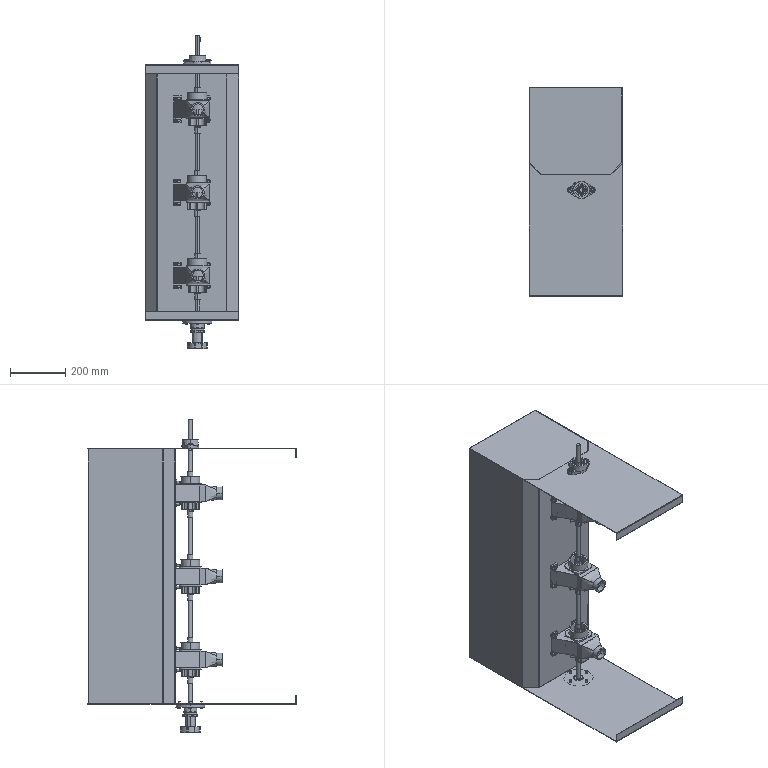Part | SolidWorks | features ReferencePattern 18, LocalLPattern 3, CompositeCurve 2, LocalCirPattern 1 | 52 solids | 1553 faces | box 338 x 752 x 1133 mm | volume 4481337 mm3 | plane 762 | cylinder 505 | cone 166 | torus 74 | spline 36 | sphere 10 | commonest cylinder face diameters 8 x56 70 x49 5 x37 25.003 x36 7 x32 13 x32